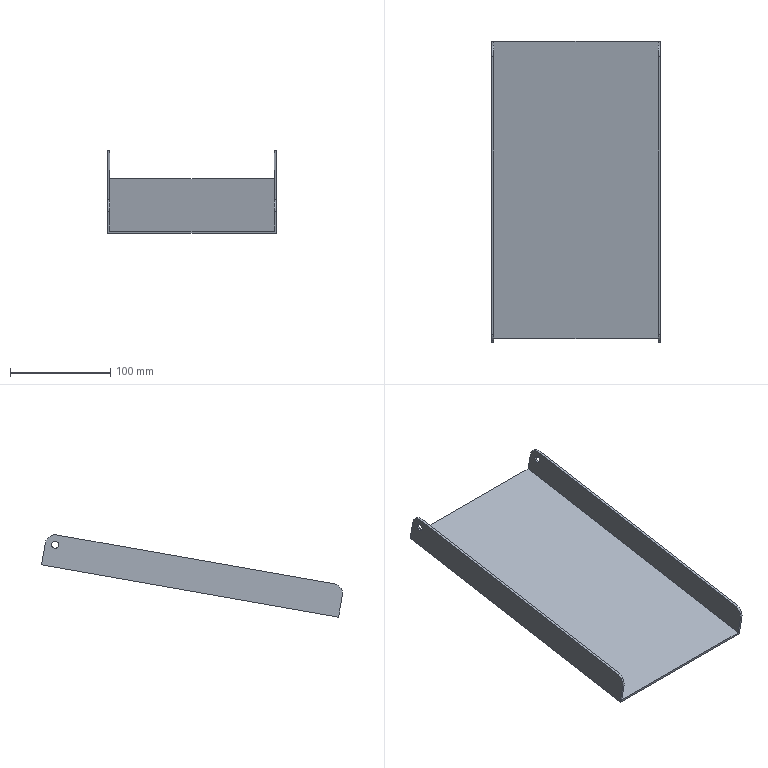Part | NX | features HB 2 | 1 solid | 16 faces | box 168 x 300.028 x 82.132 mm | volume 136758 mm3 | plane 10 | cylinder 6 | commonest cylinder face diameters 20 x4 7 x2
STEP:
#1=CARTESIAN_POINT('',(124.,-684.707,-373.956));
#2=VERTEX_POINT('',#1);
#3=CARTESIAN_POINT('',(124.,-685.612,-377.336));
#4=DIRECTION('',(1.,0.,0.));
#5=DIRECTION('',(0.,0.2588,0.9659));
#6=AXIS2_PLACEMENT_3D('',#3,#4,#5);
#7=CIRCLE('',#6,3.5);
#8=EDGE_CURVE('',#2,#2,#7,.T.);
#9=ORIENTED_EDGE('',*,*,#8,.F.);
#10=EDGE_LOOP('',(#9));
#11=FACE_BOUND('',#10,.T.);
#12=CARTESIAN_POINT('',(126.,-684.707,-373.956));
#13=VERTEX_POINT('',#12);
#14=CARTESIAN_POINT('',(126.,-685.612,-377.336));
#15=DIRECTION('',(-1.,0.,0.));
#16=DIRECTION('',(0.,0.2588,0.9659));
#17=AXIS2_PLACEMENT_3D('',#14,#15,#16);
#18=CIRCLE('',#17,3.5);
#19=EDGE_CURVE('',#13,#13,#18,.T.);
#20=ORIENTED_EDGE('',*,*,#19,.F.);
#21=EDGE_LOOP('',(#20));
#22=FACE_BOUND('',#21,.T.);
#23=CARTESIAN_POINT('',(826.,-685.612,-377.336));
#24=DIRECTION('',(-1.,0.,0.));
#25=DIRECTION('',(0.,-0.2588,-0.9659));
#26=AXIS2_PLACEMENT_3D('',#23,#24,#25);
#27=CYLINDRICAL_SURFACE('',#26,3.5);
#28=ADVANCED_FACE('',(#11,#22),#27,.F.);
#29=CARTESIAN_POINT('',(124.,-687.349,-367.488));
#30=VERTEX_POINT('',#29);
#31=CARTESIAN_POINT('',(124.,-963.709,-416.218));
#32=VERTEX_POINT('',#31);
#33=CARTESIAN_POINT('',(124.,-562.892,-345.543));
#34=DIRECTION('',(0.,-0.9848,-0.1736));
#35=VECTOR('',#34,1000.);
#36=LINE('',#33,#35);
#37=EDGE_CURVE('',#30,#32,#36,.T.);
#38=ORIENTED_EDGE('',*,*,#37,.T.);
#39=CARTESIAN_POINT('',(126.,-963.709,-416.218));
#40=VERTEX_POINT('',#39);
#41=CARTESIAN_POINT('',(220.,-963.709,-416.218));
#42=DIRECTION('',(1.,0.,0.));
#43=VECTOR('',#42,1000.);
#44=LINE('',#41,#43);
#45=EDGE_CURVE('',#32,#40,#44,.T.);
#46=ORIENTED_EDGE('',*,*,#45,.T.);
#47=CARTESIAN_POINT('',(126.,-687.349,-367.488));
#48=VERTEX_POINT('',#47);
#49=CARTESIAN_POINT('',(126.,-562.892,-345.543));
#50=DIRECTION('',(0.,-0.9848,-0.1736));
#51=VECTOR('',#50,1000.);
#52=LINE('',#49,#51);
#53=EDGE_CURVE('',#48,#40,#52,.T.);
#54=ORIENTED_EDGE('',*,*,#53,.F.);
#55=CARTESIAN_POINT('',(220.,-687.349,-367.488));
#56=DIRECTION('',(1.,0.,0.));
#57=VECTOR('',#56,1000.);
#58=LINE('',#55,#57);
#59=EDGE_CURVE('',#30,#48,#58,.T.);
#60=ORIENTED_EDGE('',*,*,#59,.F.);
#61=EDGE_LOOP('',(#38,#46,#54,#60));
#62=FACE_BOUND('',#61,.T.);
#63=CARTESIAN_POINT('',(220.,-562.892,-345.543));
#64=DIRECTION('',(0.,0.1736,-0.9848));
#65=DIRECTION('',(0.,-0.9848,-0.1736));
#66=AXIS2_PLACEMENT_3D('',#63,#64,#65);
#67=PLANE('',#66);
#68=ADVANCED_FACE('',(#62),#67,.F.);
#69=CARTESIAN_POINT('',(124.,-971.82,-427.803));
#70=VERTEX_POINT('',#69);
#71=CARTESIAN_POINT('',(124.,-961.972,-426.066));
#72=DIRECTION('',(-1.,0.,0.));
#73=DIRECTION('',(0.,0.2588,0.9659));
#74=AXIS2_PLACEMENT_3D('',#71,#72,#73);
#75=CIRCLE('',#74,10.);
#76=EDGE_CURVE('',#70,#32,#75,.T.);
#77=ORIENTED_EDGE('',*,*,#76,.F.);
#78=CARTESIAN_POINT('',(126.,-971.82,-427.803));
#79=VERTEX_POINT('',#78);
#80=CARTESIAN_POINT('',(180.,-971.82,-427.803));
#81=DIRECTION('',(-1.,0.,0.));
#82=VECTOR('',#81,1000.);
#83=LINE('',#80,#82);
#84=EDGE_CURVE('',#79,#70,#83,.T.);
#85=ORIENTED_EDGE('',*,*,#84,.F.);
#86=CARTESIAN_POINT('',(126.,-961.972,-426.066));
#87=DIRECTION('',(1.,0.,0.));
#88=DIRECTION('',(0.,0.2588,0.9659));
#89=AXIS2_PLACEMENT_3D('',#86,#87,#88);
#90=CIRCLE('',#89,10.);
#91=EDGE_CURVE('',#40,#79,#90,.T.);
#92=ORIENTED_EDGE('',*,*,#91,.F.);
#93=ORIENTED_EDGE('',*,*,#45,.F.);
#94=EDGE_LOOP('',(#77,#85,#92,#93));
#95=FACE_BOUND('',#94,.T.);
#96=CARTESIAN_POINT('',(220.,-961.972,-426.066));
#97=DIRECTION('',(1.,0.,0.));
#98=DIRECTION('',(0.,0.2588,0.9659));
#99=AXIS2_PLACEMENT_3D('',#96,#97,#98);
#100=CYLINDRICAL_SURFACE('',#99,10.);
#101=ADVANCED_FACE('',(#95),#100,.T.);
#102=ORIENTED_EDGE('',*,*,#53,.T.);
#103=ORIENTED_EDGE('',*,*,#91,.T.);
#104=CARTESIAN_POINT('',(126.,-968.,-449.468));
#105=VERTEX_POINT('',#104);
#106=CARTESIAN_POINT('',(126.,-968.347,-447.499));
#107=DIRECTION('',(0.,0.1736,-0.9848));
#108=VECTOR('',#107,1000.);
#109=LINE('',#106,#108);
#110=EDGE_CURVE('',#79,#105,#109,.T.);
#111=ORIENTED_EDGE('',*,*,#110,.T.);
#112=CARTESIAN_POINT('',(126.,-671.944,-397.266));
#113=VERTEX_POINT('',#112);
#114=CARTESIAN_POINT('',(126.,-557.335,-377.057));
#115=DIRECTION('',(0.,0.9848,0.1736));
#116=VECTOR('',#115,1000.);
#117=LINE('',#114,#116);
#118=EDGE_CURVE('',#105,#113,#117,.T.);
#119=ORIENTED_EDGE('',*,*,#118,.T.);
#120=CARTESIAN_POINT('',(126.,-675.764,-375.6));
#121=VERTEX_POINT('',#120);
#122=CARTESIAN_POINT('',(126.,-672.291,-395.296));
#123=DIRECTION('',(0.,0.1736,-0.9848));
#124=VECTOR('',#123,1000.);
#125=LINE('',#122,#124);
#126=EDGE_CURVE('',#121,#113,#125,.T.);
#127=ORIENTED_EDGE('',*,*,#126,.F.);
#128=CARTESIAN_POINT('',(126.,-685.612,-377.336));
#129=DIRECTION('',(-1.,0.,0.));
#130=DIRECTION('',(0.,-0.5736,0.8192));
#131=AXIS2_PLACEMENT_3D('',#128,#129,#130);
#132=CIRCLE('',#131,10.);
#133=EDGE_CURVE('',#48,#121,#132,.T.);
#134=ORIENTED_EDGE('',*,*,#133,.F.);
#135=EDGE_LOOP('',(#102,#103,#111,#119,#127,#134));
#136=FACE_BOUND('',#135,.T.);
#137=ORIENTED_EDGE('',*,*,#19,.T.);
#138=EDGE_LOOP('',(#137));
#139=FACE_BOUND('',#138,.T.);
#140=CARTESIAN_POINT('',(126.,-557.683,-375.087));
#141=DIRECTION('',(-1.,0.,0.));
#142=DIRECTION('',(0.,-0.2588,-0.9659));
#143=AXIS2_PLACEMENT_3D('',#140,#141,#142);
#144=PLANE('',#143);
#145=ADVANCED_FACE('',(#136,#139),#144,.F.);
#146=CARTESIAN_POINT('',(124.,-675.764,-375.6));
#147=VERTEX_POINT('',#146);
#148=CARTESIAN_POINT('',(124.,-685.612,-377.336));
#149=DIRECTION('',(1.,0.,0.));
#150=DIRECTION('',(0.,-0.5736,0.8192));
#151=AXIS2_PLACEMENT_3D('',#148,#149,#150);
#152=CIRCLE('',#151,10.);
#153=EDGE_CURVE('',#147,#30,#152,.T.);
#154=ORIENTED_EDGE('',*,*,#153,.T.);
#155=ORIENTED_EDGE('',*,*,#59,.T.);
#156=ORIENTED_EDGE('',*,*,#133,.T.);
#157=CARTESIAN_POINT('',(220.,-675.764,-375.6));
#158=DIRECTION('',(-1.,0.,0.));
#159=VECTOR('',#158,1000.);
#160=LINE('',#157,#159);
#161=EDGE_CURVE('',#121,#147,#160,.T.);
#162=ORIENTED_EDGE('',*,*,#161,.T.);
#163=EDGE_LOOP('',(#154,#155,#156,#162));
#164=FACE_BOUND('',#163,.T.);
#165=CARTESIAN_POINT('',(220.,-685.612,-377.336));
#166=DIRECTION('',(1.,0.,0.));
#167=DIRECTION('',(0.,-0.5736,0.8192));
#168=AXIS2_PLACEMENT_3D('',#165,#166,#167);
#169=CYLINDRICAL_SURFACE('',#168,10.);
#170=ADVANCED_FACE('',(#164),#169,.T.);
#171=ORIENTED_EDGE('',*,*,#76,.T.);
#172=ORIENTED_EDGE('',*,*,#37,.F.);
#173=ORIENTED_EDGE('',*,*,#153,.F.);
#174=CARTESIAN_POINT('',(124.,-672.291,-395.296));
#175=VERTEX_POINT('',#174);
#176=CARTESIAN_POINT('',(124.,-672.291,-395.296));
#177=DIRECTION('',(0.,0.1736,-0.9848));
#178=VECTOR('',#177,1000.);
#179=LINE('',#176,#178);
#180=EDGE_CURVE('',#147,#175,#179,.T.);
#181=ORIENTED_EDGE('',*,*,#180,.T.);
#182=CARTESIAN_POINT('',(124.,-968.347,-447.499));
#183=VERTEX_POINT('',#182);
#184=CARTESIAN_POINT('',(124.,-557.683,-375.087));
#185=DIRECTION('',(0.,-0.9848,-0.1736));
#186=VECTOR('',#185,1000.);
#187=LINE('',#184,#186);
#188=EDGE_CURVE('',#175,#183,#187,.T.);
#189=ORIENTED_EDGE('',*,*,#188,.T.);
#190=CARTESIAN_POINT('',(124.,-968.347,-447.499));
#191=DIRECTION('',(0.,0.1736,-0.9848));
#192=VECTOR('',#191,1000.);
#193=LINE('',#190,#192);
#194=EDGE_CURVE('',#70,#183,#193,.T.);
#195=ORIENTED_EDGE('',*,*,#194,.F.);
#196=EDGE_LOOP('',(#171,#172,#173,#181,#189,#195));
#197=FACE_BOUND('',#196,.T.);
#198=ORIENTED_EDGE('',*,*,#8,.T.);
#199=EDGE_LOOP('',(#198));
#200=FACE_BOUND('',#199,.T.);
#201=CARTESIAN_POINT('',(124.,-557.683,-375.087));
#202=DIRECTION('',(-1.,0.,0.));
#203=DIRECTION('',(0.,0.2588,0.9659));
#204=AXIS2_PLACEMENT_3D('',#201,#202,#203);
#205=PLANE('',#204);
#206=ADVANCED_FACE('',(#197,#200),#205,.T.);
#207=CARTESIAN_POINT('',(-40.,-672.291,-395.296));
#208=VERTEX_POINT('',#207);
#209=CARTESIAN_POINT('',(180.,-672.291,-395.296));
#210=DIRECTION('',(1.,0.,0.));
#211=VECTOR('',#210,1000.);
#212=LINE('',#209,#211);
#213=EDGE_CURVE('',#208,#175,#212,.T.);
#214=ORIENTED_EDGE('',*,*,#213,.T.);
#215=ORIENTED_EDGE('',*,*,#180,.F.);
#216=ORIENTED_EDGE('',*,*,#161,.F.);
#217=ORIENTED_EDGE('',*,*,#126,.T.);
#218=CARTESIAN_POINT('',(-42.,-671.944,-397.266));
#219=VERTEX_POINT('',#218);
#220=CARTESIAN_POINT('',(180.,-671.944,-397.266));
#221=DIRECTION('',(1.,0.,0.));
#222=VECTOR('',#221,1000.);
#223=LINE('',#220,#222);
#224=EDGE_CURVE('',#219,#113,#223,.T.);
#225=ORIENTED_EDGE('',*,*,#224,.F.);
#226=CARTESIAN_POINT('',(-42.,-675.764,-375.6));
#227=VERTEX_POINT('',#226);
#228=CARTESIAN_POINT('',(-42.,-672.291,-395.296));
#229=DIRECTION('',(0.,0.1736,-0.9848));
#230=VECTOR('',#229,1000.);
#231=LINE('',#228,#230);
#232=EDGE_CURVE('',#227,#219,#231,.T.);
#233=ORIENTED_EDGE('',*,*,#232,.F.);
#234=CARTESIAN_POINT('',(-40.,-675.764,-375.6));
#235=VERTEX_POINT('',#234);
#236=CARTESIAN_POINT('',(263.,-675.764,-375.6));
#237=DIRECTION('',(-1.,0.,0.));
#238=VECTOR('',#237,1000.);
#239=LINE('',#236,#238);
#240=EDGE_CURVE('',#235,#227,#239,.T.);
#241=ORIENTED_EDGE('',*,*,#240,.F.);
#242=CARTESIAN_POINT('',(-40.,-672.291,-395.296));
#243=DIRECTION('',(0.,0.1736,-0.9848));
#244=VECTOR('',#243,1000.);
#245=LINE('',#242,#244);
#246=EDGE_CURVE('',#235,#208,#245,.T.);
#247=ORIENTED_EDGE('',*,*,#246,.T.);
#248=EDGE_LOOP('',(#214,#215,#216,#217,#225,#233,#241,#247));
#249=FACE_BOUND('',#248,.T.);
#250=CARTESIAN_POINT('',(180.,-672.291,-395.296));
#251=DIRECTION('',(0.,-0.9848,-0.1736));
#252=DIRECTION('',(0.,0.1736,-0.9848));
#253=AXIS2_PLACEMENT_3D('',#250,#251,#252);
#254=PLANE('',#253);
#255=ADVANCED_FACE('',(#249),#254,.F.);
#256=ORIENTED_EDGE('',*,*,#194,.T.);
#257=CARTESIAN_POINT('',(-40.,-968.347,-447.499));
#258=VERTEX_POINT('',#257);
#259=CARTESIAN_POINT('',(180.,-968.347,-447.499));
#260=DIRECTION('',(1.,0.,0.));
#261=VECTOR('',#260,1000.);
#262=LINE('',#259,#261);
#263=EDGE_CURVE('',#258,#183,#262,.T.);
#264=ORIENTED_EDGE('',*,*,#263,.F.);
#265=CARTESIAN_POINT('',(-40.,-971.82,-427.803));
#266=VERTEX_POINT('',#265);
#267=CARTESIAN_POINT('',(-40.,-968.347,-447.499));
#268=DIRECTION('',(0.,0.1736,-0.9848));
#269=VECTOR('',#268,1000.);
#270=LINE('',#267,#269);
#271=EDGE_CURVE('',#266,#258,#270,.T.);
#272=ORIENTED_EDGE('',*,*,#271,.F.);
#273=CARTESIAN_POINT('',(-42.,-971.82,-427.803));
#274=VERTEX_POINT('',#273);
#275=CARTESIAN_POINT('',(180.,-971.82,-427.803));
#276=DIRECTION('',(-1.,0.,0.));
#277=VECTOR('',#276,1000.);
#278=LINE('',#275,#277);
#279=EDGE_CURVE('',#266,#274,#278,.T.);
#280=ORIENTED_EDGE('',*,*,#279,.T.);
#281=CARTESIAN_POINT('',(-42.,-968.,-449.468));
#282=VERTEX_POINT('',#281);
#283=CARTESIAN_POINT('',(-42.,-968.347,-447.499));
#284=DIRECTION('',(0.,0.1736,-0.9848));
#285=VECTOR('',#284,1000.);
#286=LINE('',#283,#285);
#287=EDGE_CURVE('',#274,#282,#286,.T.);
#288=ORIENTED_EDGE('',*,*,#287,.T.);
#289=CARTESIAN_POINT('',(180.,-968.,-449.468));
#290=DIRECTION('',(1.,0.,0.));
#291=VECTOR('',#290,1000.);
#292=LINE('',#289,#291);
#293=EDGE_CURVE('',#282,#105,#292,.T.);
#294=ORIENTED_EDGE('',*,*,#293,.T.);
#295=ORIENTED_EDGE('',*,*,#110,.F.);
#296=ORIENTED_EDGE('',*,*,#84,.T.);
#297=EDGE_LOOP('',(#256,#264,#272,#280,#288,#294,#295,#296));
#298=FACE_BOUND('',#297,.T.);
#299=CARTESIAN_POINT('',(180.,-968.347,-447.499));
#300=DIRECTION('',(0.,0.9848,0.1736));
#301=DIRECTION('',(0.,0.1736,-0.9848));
#302=AXIS2_PLACEMENT_3D('',#299,#300,#301);
#303=PLANE('',#302);
#304=ADVANCED_FACE('',(#298),#303,.F.);
#305=ORIENTED_EDGE('',*,*,#118,.F.);
#306=ORIENTED_EDGE('',*,*,#293,.F.);
#307=CARTESIAN_POINT('',(-42.,-557.335,-377.057));
#308=DIRECTION('',(0.,-0.9848,-0.1736));
#309=VECTOR('',#308,1000.);
#310=LINE('',#307,#309);
#311=EDGE_CURVE('',#219,#282,#310,.T.);
#312=ORIENTED_EDGE('',*,*,#311,.F.);
#313=ORIENTED_EDGE('',*,*,#224,.T.);
#314=EDGE_LOOP('',(#305,#306,#312,#313));
#315=FACE_BOUND('',#314,.T.);
#316=CARTESIAN_POINT('',(180.,-557.335,-377.057));
#317=DIRECTION('',(0.,-0.1736,0.9848));
#318=DIRECTION('',(-1.,0.,0.));
#319=AXIS2_PLACEMENT_3D('',#316,#317,#318);
#320=PLANE('',#319);
#321=ADVANCED_FACE('',(#315),#320,.F.);
#322=ORIENTED_EDGE('',*,*,#263,.T.);
#323=ORIENTED_EDGE('',*,*,#188,.F.);
#324=ORIENTED_EDGE('',*,*,#213,.F.);
#325=CARTESIAN_POINT('',(-40.,-557.683,-375.087));
#326=DIRECTION('',(0.,0.9848,0.1736));
#327=VECTOR('',#326,1000.);
#328=LINE('',#325,#327);
#329=EDGE_CURVE('',#258,#208,#328,.T.);
#330=ORIENTED_EDGE('',*,*,#329,.F.);
#331=EDGE_LOOP('',(#322,#323,#324,#330));
#332=FACE_BOUND('',#331,.T.);
#333=CARTESIAN_POINT('',(180.,-557.683,-375.087));
#334=DIRECTION('',(0.,-0.1736,0.9848));
#335=DIRECTION('',(-1.,0.,0.));
#336=AXIS2_PLACEMENT_3D('',#333,#334,#335);
#337=PLANE('',#336);
#338=ADVANCED_FACE('',(#332),#337,.T.);
#339=CARTESIAN_POINT('',(-42.,-686.518,-380.717));
#340=VERTEX_POINT('',#339);
#341=CARTESIAN_POINT('',(-42.,-685.612,-377.336));
#342=DIRECTION('',(1.,0.,0.));
#343=DIRECTION('',(0.,-0.2588,-0.9659));
#344=AXIS2_PLACEMENT_3D('',#341,#342,#343);
#345=CIRCLE('',#344,3.5);
#346=EDGE_CURVE('',#340,#340,#345,.T.);
#347=ORIENTED_EDGE('',*,*,#346,.T.);
#348=EDGE_LOOP('',(#347));
#349=FACE_BOUND('',#348,.T.);
#350=ORIENTED_EDGE('',*,*,#311,.T.);
#351=ORIENTED_EDGE('',*,*,#287,.F.);
#352=CARTESIAN_POINT('',(-42.,-963.709,-416.218));
#353=VERTEX_POINT('',#352);
#354=CARTESIAN_POINT('',(-42.,-961.972,-426.066));
#355=DIRECTION('',(-1.,0.,0.));
#356=DIRECTION('',(0.,-0.2588,-0.9659));
#357=AXIS2_PLACEMENT_3D('',#354,#355,#356);
#358=CIRCLE('',#357,10.);
#359=EDGE_CURVE('',#274,#353,#358,.T.);
#360=ORIENTED_EDGE('',*,*,#359,.T.);
#361=CARTESIAN_POINT('',(-42.,-687.349,-367.488));
#362=VERTEX_POINT('',#361);
#363=CARTESIAN_POINT('',(-42.,-562.892,-345.543));
#364=DIRECTION('',(0.,-0.9848,-0.1736));
#365=VECTOR('',#364,1000.);
#366=LINE('',#363,#365);
#367=EDGE_CURVE('',#362,#353,#366,.T.);
#368=ORIENTED_EDGE('',*,*,#367,.F.);
#369=CARTESIAN_POINT('',(-42.,-685.612,-377.336));
#370=DIRECTION('',(1.,0.,0.));
#371=DIRECTION('',(0.,0.5736,-0.8192));
#372=AXIS2_PLACEMENT_3D('',#369,#370,#371);
#373=CIRCLE('',#372,10.);
#374=EDGE_CURVE('',#227,#362,#373,.T.);
#375=ORIENTED_EDGE('',*,*,#374,.F.);
#376=ORIENTED_EDGE('',*,*,#232,.T.);
#377=EDGE_LOOP('',(#350,#351,#360,#368,#375,#376));
#378=FACE_BOUND('',#377,.T.);
#379=CARTESIAN_POINT('',(-42.,-557.683,-375.087));
#380=DIRECTION('',(1.,0.,0.));
#381=DIRECTION('',(0.,0.2588,0.9659));
#382=AXIS2_PLACEMENT_3D('',#379,#380,#381);
#383=PLANE('',#382);
#384=ADVANCED_FACE('',(#349,#378),#383,.F.);
#385=ORIENTED_EDGE('',*,*,#367,.T.);
#386=CARTESIAN_POINT('',(-40.,-963.709,-416.218));
#387=VERTEX_POINT('',#386);
#388=CARTESIAN_POINT('',(5.,-963.709,-416.218));
#389=DIRECTION('',(1.,0.,0.));
#390=VECTOR('',#389,1000.);
#391=LINE('',#388,#390);
#392=EDGE_CURVE('',#353,#387,#391,.T.);
#393=ORIENTED_EDGE('',*,*,#392,.T.);
#394=CARTESIAN_POINT('',(-40.,-687.349,-367.488));
#395=VERTEX_POINT('',#394);
#396=CARTESIAN_POINT('',(-40.,-562.892,-345.543));
#397=DIRECTION('',(0.,-0.9848,-0.1736));
#398=VECTOR('',#397,1000.);
#399=LINE('',#396,#398);
#400=EDGE_CURVE('',#395,#387,#399,.T.);
#401=ORIENTED_EDGE('',*,*,#400,.F.);
#402=CARTESIAN_POINT('',(5.,-687.349,-367.488));
#403=DIRECTION('',(1.,0.,0.));
#404=VECTOR('',#403,1000.);
#405=LINE('',#402,#404);
#406=EDGE_CURVE('',#362,#395,#405,.T.);
#407=ORIENTED_EDGE('',*,*,#406,.F.);
#408=EDGE_LOOP('',(#385,#393,#401,#407));
#409=FACE_BOUND('',#408,.T.);
#410=CARTESIAN_POINT('',(5.,-562.892,-345.543));
#411=DIRECTION('',(0.,0.1736,-0.9848));
#412=DIRECTION('',(0.,-0.9848,-0.1736));
#413=AXIS2_PLACEMENT_3D('',#410,#411,#412);
#414=PLANE('',#413);
#415=ADVANCED_FACE('',(#409),#414,.F.);
#416=CARTESIAN_POINT('',(-40.,-686.518,-380.717));
#417=VERTEX_POINT('',#416);
#418=CARTESIAN_POINT('',(-40.,-685.612,-377.336));
#419=DIRECTION('',(1.,0.,0.));
#420=DIRECTION('',(0.,-0.2588,-0.9659));
#421=AXIS2_PLACEMENT_3D('',#418,#419,#420);
#422=CIRCLE('',#421,3.5);
#423=EDGE_CURVE('',#417,#417,#422,.T.);
#424=ORIENTED_EDGE('',*,*,#423,.F.);
#425=EDGE_LOOP('',(#424));
#426=FACE_BOUND('',#425,.T.);
#427=ORIENTED_EDGE('',*,*,#329,.T.);
#428=ORIENTED_EDGE('',*,*,#246,.F.);
#429=CARTESIAN_POINT('',(-40.,-685.612,-377.336));
#430=DIRECTION('',(-1.,0.,0.));
#431=DIRECTION('',(0.,0.5736,-0.8192));
#432=AXIS2_PLACEMENT_3D('',#429,#430,#431);
#433=CIRCLE('',#432,10.);
#434=EDGE_CURVE('',#395,#235,#433,.T.);
#435=ORIENTED_EDGE('',*,*,#434,.F.);
#436=ORIENTED_EDGE('',*,*,#400,.T.);
#437=CARTESIAN_POINT('',(-40.,-961.972,-426.066));
#438=DIRECTION('',(1.,0.,0.));
#439=DIRECTION('',(0.,-0.2588,-0.9659));
#440=AXIS2_PLACEMENT_3D('',#437,#438,#439);
#441=CIRCLE('',#440,10.);
#442=EDGE_CURVE('',#387,#266,#441,.T.);
#443=ORIENTED_EDGE('',*,*,#442,.T.);
#444=ORIENTED_EDGE('',*,*,#271,.T.);
#445=EDGE_LOOP('',(#427,#428,#435,#436,#443,#444));
#446=FACE_BOUND('',#445,.T.);
#447=CARTESIAN_POINT('',(-40.,-557.683,-375.087));
#448=DIRECTION('',(1.,0.,0.));
#449=DIRECTION('',(0.,0.2588,0.9659));
#450=AXIS2_PLACEMENT_3D('',#447,#448,#449);
#451=PLANE('',#450);
#452=ADVANCED_FACE('',(#426,#446),#451,.T.);
#453=ORIENTED_EDGE('',*,*,#442,.F.);
#454=ORIENTED_EDGE('',*,*,#392,.F.);
#455=ORIENTED_EDGE('',*,*,#359,.F.);
#456=ORIENTED_EDGE('',*,*,#279,.F.);
#457=EDGE_LOOP('',(#453,#454,#455,#456));
#458=FACE_BOUND('',#457,.T.);
#459=CARTESIAN_POINT('',(263.,-961.972,-426.066));
#460=DIRECTION('',(-1.,0.,0.));
#461=DIRECTION('',(0.,-0.2588,-0.9659));
#462=AXIS2_PLACEMENT_3D('',#459,#460,#461);
#463=CYLINDRICAL_SURFACE('',#462,10.);
#464=ADVANCED_FACE('',(#458),#463,.T.);
#465=ORIENTED_EDGE('',*,*,#434,.T.);
#466=ORIENTED_EDGE('',*,*,#240,.T.);
#467=ORIENTED_EDGE('',*,*,#374,.T.);
#468=ORIENTED_EDGE('',*,*,#406,.T.);
#469=EDGE_LOOP('',(#465,#466,#467,#468));
#470=FACE_BOUND('',#469,.T.);
#471=CARTESIAN_POINT('',(263.,-685.612,-377.336));
#472=DIRECTION('',(-1.,0.,0.));
#473=DIRECTION('',(0.,0.5736,-0.8192));
#474=AXIS2_PLACEMENT_3D('',#471,#472,#473);
#475=CYLINDRICAL_SURFACE('',#474,10.);
#476=ADVANCED_FACE('',(#470),#475,.T.);
#477=ORIENTED_EDGE('',*,*,#423,.T.);
#478=EDGE_LOOP('',(#477));
#479=FACE_BOUND('',#478,.T.);
#480=ORIENTED_EDGE('',*,*,#346,.F.);
#481=EDGE_LOOP('',(#480));
#482=FACE_BOUND('',#481,.T.);
#483=CARTESIAN_POINT('',(3.,-685.612,-377.336));
#484=DIRECTION('',(1.,0.,0.));
#485=DIRECTION('',(0.,0.2588,0.9659));
#486=AXIS2_PLACEMENT_3D('',#483,#484,#485);
#487=CYLINDRICAL_SURFACE('',#486,3.5);
#488=ADVANCED_FACE('',(#479,#482),#487,.F.);
#489=CLOSED_SHELL('',(#28,#68,#101,#145,#170,#206,#255,#304,#321,#338,#384,#415,#452,#464,#476,#488));
#490=MANIFOLD_SOLID_BREP('',#489);
#491=(LENGTH_UNIT()NAMED_UNIT(*)SI_UNIT(.MILLI.,.METRE.));
#492=UNCERTAINTY_MEASURE_WITH_UNIT(LENGTH_MEASURE(0.00001),#491,'','');
#493=(NAMED_UNIT(*)PLANE_ANGLE_UNIT()SI_UNIT($,.RADIAN.));
#494=(NAMED_UNIT(*)SI_UNIT($,.STERADIAN.)SOLID_ANGLE_UNIT());
#495=(GEOMETRIC_REPRESENTATION_CONTEXT(3)GLOBAL_UNCERTAINTY_ASSIGNED_CONTEXT((#492))GLOBAL_UNIT_ASSIGNED_CONTEXT((#491,#493,#494))REPRESENTATION_CONTEXT('',''));
#496=ADVANCED_BREP_SHAPE_REPRESENTATION('',(#490),#495);